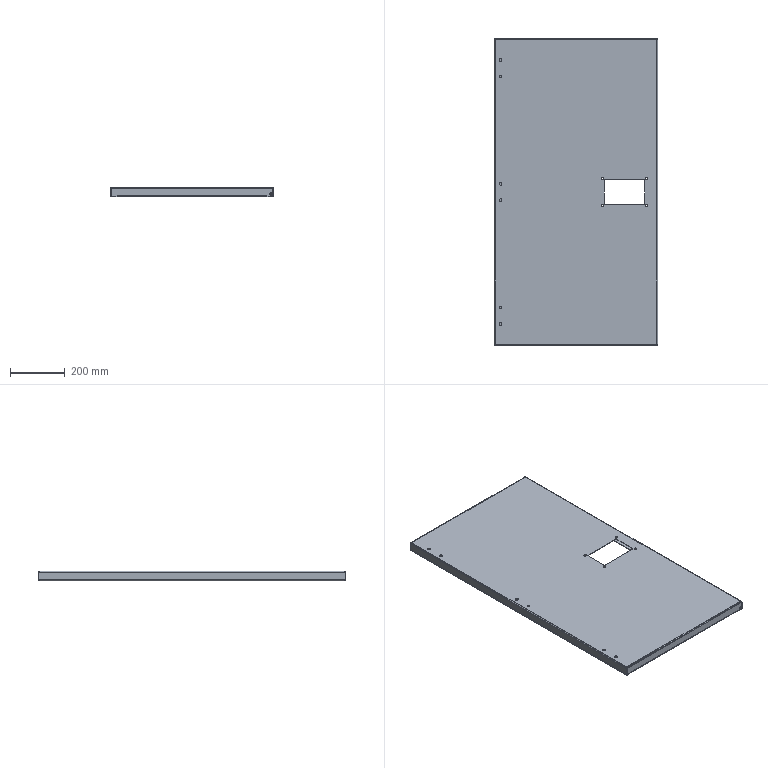Part | STEP file | SYL_0392D6J1SYL0380DJ100-623151 | 1 solid | 130 faces | box 594 x 1114 x 35 mm | volume 1655026 mm3 | plane 78 | cylinder 44 | spline 8 | commonest cylinder face diameters 8 x12 10.5 x12 4 x8 9 x8 6 x4